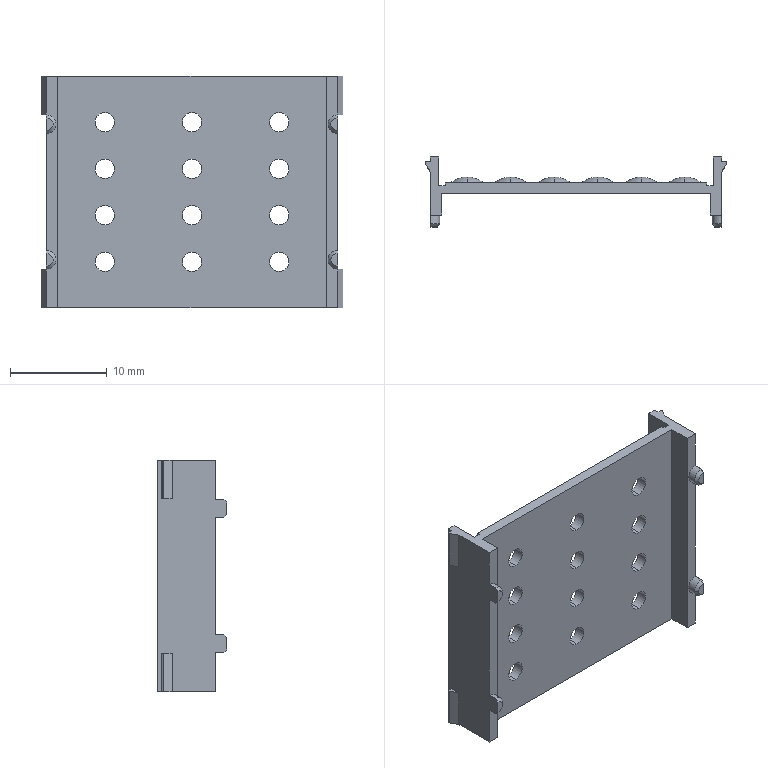Part | SolidWorks | features BaseBody 1 | 1 solid | 148 faces | box 31.173 x 7.2 x 23.95 mm | volume 1073 mm3 | spline 60 | cylinder 41 | plane 34 | cone 13 | commonest cylinder face diameters 2 x24 1.9 x12 0.2 x5